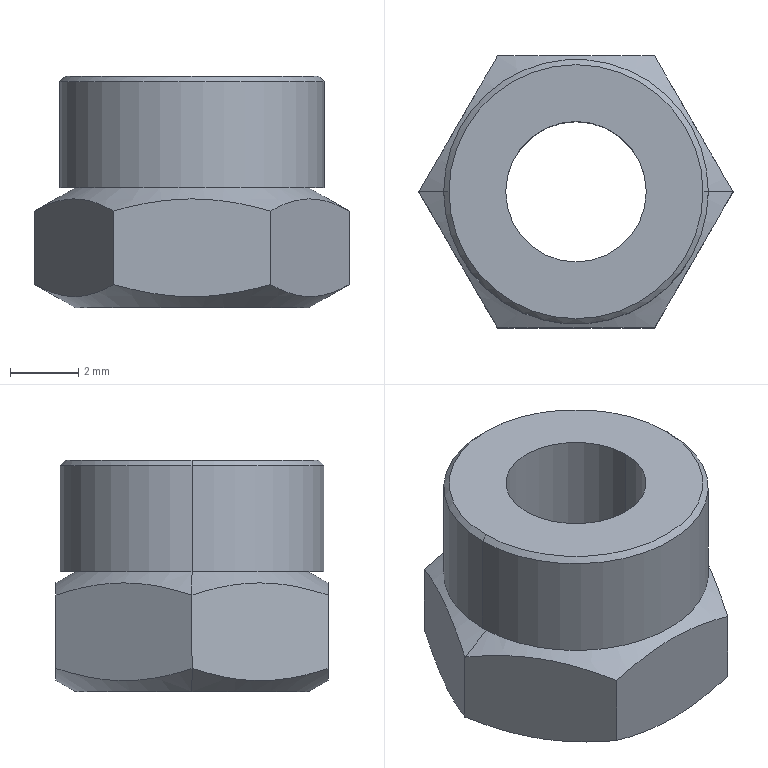Part | STEP file | prevailing torque type style 1 gbV1.201001_GB_HEXAGON_TYPE9 M5-N | 1 solid | 21 faces | box 9.238 x 8 x 6.8 mm | volume 245.877 mm3 | plane 9 | cone 8 | cylinder 4 | commonest cylinder face diameters 4.134 x2 7.78 x2